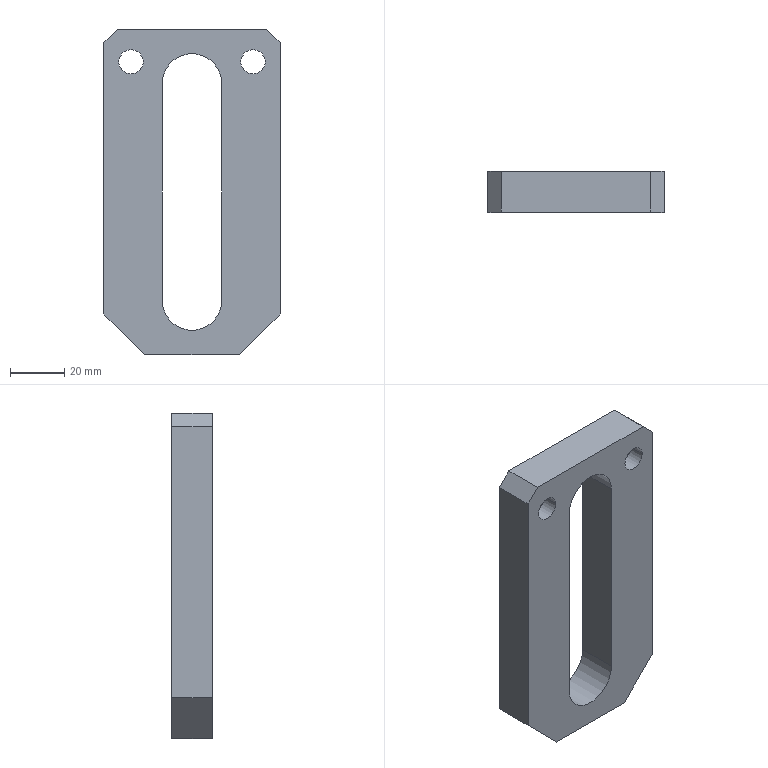Part | NX | features 001 2 | 1 solid | 24 faces | box 65 x 15 x 120 mm | volume 77204 mm3 | plane 14 | cylinder 10 | commonest cylinder face diameters 9 x4 15 x4 22 x2
STEP:
#1=CARTESIAN_POINT('',(114.773,73.,14.));
#2=VERTEX_POINT('',#1);
#3=CARTESIAN_POINT('',(114.773,58.,14.));
#4=VERTEX_POINT('',#3);
#5=CARTESIAN_POINT('',(114.773,73.,14.));
#6=DIRECTION('',(0.,-1.,0.));
#7=VECTOR('',#6,1000.);
#8=LINE('',#5,#7);
#9=EDGE_CURVE('',#2,#4,#8,.T.);
#10=ORIENTED_EDGE('',*,*,#9,.F.);
#11=CARTESIAN_POINT('',(114.773,73.,-66.));
#12=VERTEX_POINT('',#11);
#13=CARTESIAN_POINT('',(114.773,73.,-66.));
#14=DIRECTION('',(0.,0.,1.));
#15=VECTOR('',#14,1000.);
#16=LINE('',#13,#15);
#17=EDGE_CURVE('',#12,#2,#16,.T.);
#18=ORIENTED_EDGE('',*,*,#17,.F.);
#19=CARTESIAN_POINT('',(114.773,58.,-66.));
#20=VERTEX_POINT('',#19);
#21=CARTESIAN_POINT('',(114.773,58.,-66.));
#22=DIRECTION('',(0.,1.,0.));
#23=VECTOR('',#22,1000.);
#24=LINE('',#21,#23);
#25=EDGE_CURVE('',#20,#12,#24,.T.);
#26=ORIENTED_EDGE('',*,*,#25,.F.);
#27=CARTESIAN_POINT('',(114.773,58.,-66.));
#28=DIRECTION('',(0.,0.,1.));
#29=VECTOR('',#28,1000.);
#30=LINE('',#27,#29);
#31=EDGE_CURVE('',#20,#4,#30,.T.);
#32=ORIENTED_EDGE('',*,*,#31,.T.);
#33=EDGE_LOOP('',(#10,#18,#26,#32));
#34=FACE_BOUND('',#33,.T.);
#35=CARTESIAN_POINT('',(114.773,73.,-66.));
#36=DIRECTION('',(-1.,0.,0.));
#37=DIRECTION('',(0.,-1.,0.));
#38=AXIS2_PLACEMENT_3D('',#35,#36,#37);
#39=PLANE('',#38);
#40=ADVANCED_FACE('',(#34),#39,.T.);
#41=CARTESIAN_POINT('',(92.773,58.,14.));
#42=VERTEX_POINT('',#41);
#43=CARTESIAN_POINT('',(92.773,73.,14.));
#44=VERTEX_POINT('',#43);
#45=CARTESIAN_POINT('',(92.773,58.,14.));
#46=DIRECTION('',(0.,1.,0.));
#47=VECTOR('',#46,1000.);
#48=LINE('',#45,#47);
#49=EDGE_CURVE('',#42,#44,#48,.T.);
#50=ORIENTED_EDGE('',*,*,#49,.T.);
#51=CARTESIAN_POINT('',(103.773,73.,14.));
#52=DIRECTION('',(0.,-1.,0.));
#53=DIRECTION('',(1.,0.,0.));
#54=AXIS2_PLACEMENT_3D('',#51,#52,#53);
#55=CIRCLE('',#54,11.);
#56=EDGE_CURVE('',#2,#44,#55,.T.);
#57=ORIENTED_EDGE('',*,*,#56,.F.);
#58=ORIENTED_EDGE('',*,*,#9,.T.);
#59=CARTESIAN_POINT('',(103.773,58.,14.));
#60=DIRECTION('',(0.,1.,0.));
#61=DIRECTION('',(-1.,0.,0.));
#62=AXIS2_PLACEMENT_3D('',#59,#60,#61);
#63=CIRCLE('',#62,11.);
#64=EDGE_CURVE('',#42,#4,#63,.T.);
#65=ORIENTED_EDGE('',*,*,#64,.F.);
#66=EDGE_LOOP('',(#50,#57,#58,#65));
#67=FACE_BOUND('',#66,.T.);
#68=CARTESIAN_POINT('',(103.773,73.,14.));
#69=DIRECTION('',(0.,-1.,0.));
#70=DIRECTION('',(1.,0.,0.));
#71=AXIS2_PLACEMENT_3D('',#68,#69,#70);
#72=CYLINDRICAL_SURFACE('',#71,11.);
#73=ADVANCED_FACE('',(#67),#72,.F.);
#74=CARTESIAN_POINT('',(92.773,73.,-66.));
#75=VERTEX_POINT('',#74);
#76=CARTESIAN_POINT('',(92.773,58.,-66.));
#77=VERTEX_POINT('',#76);
#78=CARTESIAN_POINT('',(92.773,73.,-66.));
#79=DIRECTION('',(0.,-1.,0.));
#80=VECTOR('',#79,1000.);
#81=LINE('',#78,#80);
#82=EDGE_CURVE('',#75,#77,#81,.T.);
#83=ORIENTED_EDGE('',*,*,#82,.F.);
#84=CARTESIAN_POINT('',(92.773,73.,14.));
#85=DIRECTION('',(0.,0.,-1.));
#86=VECTOR('',#85,1000.);
#87=LINE('',#84,#86);
#88=EDGE_CURVE('',#44,#75,#87,.T.);
#89=ORIENTED_EDGE('',*,*,#88,.F.);
#90=ORIENTED_EDGE('',*,*,#49,.F.);
#91=CARTESIAN_POINT('',(92.773,58.,14.));
#92=DIRECTION('',(0.,0.,-1.));
#93=VECTOR('',#92,1000.);
#94=LINE('',#91,#93);
#95=EDGE_CURVE('',#42,#77,#94,.T.);
#96=ORIENTED_EDGE('',*,*,#95,.T.);
#97=EDGE_LOOP('',(#83,#89,#90,#96));
#98=FACE_BOUND('',#97,.T.);
#99=CARTESIAN_POINT('',(92.773,73.,-66.));
#100=DIRECTION('',(1.,0.,0.));
#101=DIRECTION('',(0.,1.,0.));
#102=AXIS2_PLACEMENT_3D('',#99,#100,#101);
#103=PLANE('',#102);
#104=ADVANCED_FACE('',(#98),#103,.T.);
#105=ORIENTED_EDGE('',*,*,#25,.T.);
#106=CARTESIAN_POINT('',(103.773,73.,-66.));
#107=DIRECTION('',(0.,-1.,0.));
#108=DIRECTION('',(-1.,0.,0.));
#109=AXIS2_PLACEMENT_3D('',#106,#107,#108);
#110=CIRCLE('',#109,11.);
#111=EDGE_CURVE('',#75,#12,#110,.T.);
#112=ORIENTED_EDGE('',*,*,#111,.F.);
#113=ORIENTED_EDGE('',*,*,#82,.T.);
#114=CARTESIAN_POINT('',(103.773,58.,-66.));
#115=DIRECTION('',(0.,1.,0.));
#116=DIRECTION('',(1.,0.,0.));
#117=AXIS2_PLACEMENT_3D('',#114,#115,#116);
#118=CIRCLE('',#117,11.);
#119=EDGE_CURVE('',#20,#77,#118,.T.);
#120=ORIENTED_EDGE('',*,*,#119,.F.);
#121=EDGE_LOOP('',(#105,#112,#113,#120));
#122=FACE_BOUND('',#121,.T.);
#123=CARTESIAN_POINT('',(103.773,73.,-66.));
#124=DIRECTION('',(0.,-1.,0.));
#125=DIRECTION('',(1.,0.,0.));
#126=AXIS2_PLACEMENT_3D('',#123,#124,#125);
#127=CYLINDRICAL_SURFACE('',#126,11.);
#128=ADVANCED_FACE('',(#122),#127,.F.);
#129=CARTESIAN_POINT('',(88.773,64.,22.));
#130=VERTEX_POINT('',#129);
#131=CARTESIAN_POINT('',(88.773,73.,22.));
#132=VERTEX_POINT('',#131);
#133=CARTESIAN_POINT('',(88.773,73.,22.));
#134=DIRECTION('',(0.,-1.,0.));
#135=VECTOR('',#134,1000.);
#136=LINE('',#133,#135);
#137=EDGE_CURVE('',#130,#132,#136,.F.);
#138=ORIENTED_EDGE('',*,*,#137,.T.);
#139=CARTESIAN_POINT('',(73.773,73.,22.));
#140=VERTEX_POINT('',#139);
#141=CARTESIAN_POINT('',(81.273,73.,22.));
#142=DIRECTION('',(0.,-1.,0.));
#143=DIRECTION('',(-1.,0.,0.));
#144=AXIS2_PLACEMENT_3D('',#141,#142,#143);
#145=CIRCLE('',#144,7.5);
#146=EDGE_CURVE('',#140,#132,#145,.T.);
#147=ORIENTED_EDGE('',*,*,#146,.F.);
#148=CARTESIAN_POINT('',(73.773,64.,22.));
#149=VERTEX_POINT('',#148);
#150=CARTESIAN_POINT('',(73.773,73.,22.));
#151=DIRECTION('',(0.,-1.,0.));
#152=VECTOR('',#151,1000.);
#153=LINE('',#150,#152);
#154=EDGE_CURVE('',#140,#149,#153,.T.);
#155=ORIENTED_EDGE('',*,*,#154,.T.);
#156=CARTESIAN_POINT('',(81.273,64.,22.));
#157=DIRECTION('',(0.,1.,0.));
#158=DIRECTION('',(1.,0.,0.));
#159=AXIS2_PLACEMENT_3D('',#156,#157,#158);
#160=CIRCLE('',#159,7.5);
#161=EDGE_CURVE('',#130,#149,#160,.T.);
#162=ORIENTED_EDGE('',*,*,#161,.F.);
#163=EDGE_LOOP('',(#138,#147,#155,#162));
#164=FACE_BOUND('',#163,.T.);
#165=CARTESIAN_POINT('',(81.273,73.,22.));
#166=DIRECTION('',(0.,1.,0.));
#167=DIRECTION('',(-1.,0.,0.));
#168=AXIS2_PLACEMENT_3D('',#165,#166,#167);
#169=CYLINDRICAL_SURFACE('',#168,7.5);
#170=ADVANCED_FACE('',(#164),#169,.F.);
#171=CARTESIAN_POINT('',(81.273,64.,22.));
#172=DIRECTION('',(0.,1.,0.));
#173=DIRECTION('',(-1.,0.,0.));
#174=AXIS2_PLACEMENT_3D('',#171,#172,#173);
#175=CIRCLE('',#174,7.5);
#176=EDGE_CURVE('',#149,#130,#175,.T.);
#177=ORIENTED_EDGE('',*,*,#176,.F.);
#178=ORIENTED_EDGE('',*,*,#154,.F.);
#179=CARTESIAN_POINT('',(81.273,73.,22.));
#180=DIRECTION('',(0.,-1.,0.));
#181=DIRECTION('',(1.,0.,0.));
#182=AXIS2_PLACEMENT_3D('',#179,#180,#181);
#183=CIRCLE('',#182,7.5);
#184=EDGE_CURVE('',#132,#140,#183,.T.);
#185=ORIENTED_EDGE('',*,*,#184,.F.);
#186=ORIENTED_EDGE('',*,*,#137,.F.);
#187=EDGE_LOOP('',(#177,#178,#185,#186));
#188=FACE_BOUND('',#187,.T.);
#189=CARTESIAN_POINT('',(81.273,73.,22.));
#190=DIRECTION('',(0.,1.,0.));
#191=DIRECTION('',(-1.,0.,0.));
#192=AXIS2_PLACEMENT_3D('',#189,#190,#191);
#193=CYLINDRICAL_SURFACE('',#192,7.5);
#194=ADVANCED_FACE('',(#188),#193,.F.);
#195=CARTESIAN_POINT('',(76.773,64.,22.));
#196=VERTEX_POINT('',#195);
#197=CARTESIAN_POINT('',(85.773,64.,22.));
#198=VERTEX_POINT('',#197);
#199=CARTESIAN_POINT('',(81.273,64.,22.));
#200=DIRECTION('',(0.,-1.,0.));
#201=DIRECTION('',(-1.,0.,0.));
#202=AXIS2_PLACEMENT_3D('',#199,#200,#201);
#203=CIRCLE('',#202,4.5);
#204=EDGE_CURVE('',#196,#198,#203,.T.);
#205=ORIENTED_EDGE('',*,*,#204,.T.);
#206=CARTESIAN_POINT('',(81.273,64.,22.));
#207=DIRECTION('',(0.,-1.,0.));
#208=DIRECTION('',(1.,0.,0.));
#209=AXIS2_PLACEMENT_3D('',#206,#207,#208);
#210=CIRCLE('',#209,4.5);
#211=EDGE_CURVE('',#198,#196,#210,.T.);
#212=ORIENTED_EDGE('',*,*,#211,.T.);
#213=EDGE_LOOP('',(#205,#212));
#214=FACE_BOUND('',#213,.T.);
#215=ORIENTED_EDGE('',*,*,#161,.T.);
#216=ORIENTED_EDGE('',*,*,#176,.T.);
#217=EDGE_LOOP('',(#215,#216));
#218=FACE_BOUND('',#217,.T.);
#219=CARTESIAN_POINT('',(76.773,64.,22.));
#220=DIRECTION('',(0.,-1.,0.));
#221=DIRECTION('',(1.,0.,0.));
#222=AXIS2_PLACEMENT_3D('',#219,#220,#221);
#223=PLANE('',#222);
#224=ADVANCED_FACE('',(#214,#218),#223,.F.);
#225=CARTESIAN_POINT('',(85.773,58.,22.));
#226=VERTEX_POINT('',#225);
#227=CARTESIAN_POINT('',(85.773,64.,22.));
#228=DIRECTION('',(0.,-1.,0.));
#229=VECTOR('',#228,1000.);
#230=LINE('',#227,#229);
#231=EDGE_CURVE('',#226,#198,#230,.F.);
#232=ORIENTED_EDGE('',*,*,#231,.T.);
#233=ORIENTED_EDGE('',*,*,#204,.F.);
#234=CARTESIAN_POINT('',(76.773,58.,22.));
#235=VERTEX_POINT('',#234);
#236=CARTESIAN_POINT('',(76.773,64.,22.));
#237=DIRECTION('',(0.,-1.,0.));
#238=VECTOR('',#237,1000.);
#239=LINE('',#236,#238);
#240=EDGE_CURVE('',#196,#235,#239,.T.);
#241=ORIENTED_EDGE('',*,*,#240,.T.);
#242=CARTESIAN_POINT('',(81.273,58.,22.));
#243=DIRECTION('',(0.,1.,0.));
#244=DIRECTION('',(1.,0.,0.));
#245=AXIS2_PLACEMENT_3D('',#242,#243,#244);
#246=CIRCLE('',#245,4.5);
#247=EDGE_CURVE('',#226,#235,#246,.T.);
#248=ORIENTED_EDGE('',*,*,#247,.F.);
#249=EDGE_LOOP('',(#232,#233,#241,#248));
#250=FACE_BOUND('',#249,.T.);
#251=CARTESIAN_POINT('',(81.273,73.,22.));
#252=DIRECTION('',(0.,1.,0.));
#253=DIRECTION('',(-1.,0.,0.));
#254=AXIS2_PLACEMENT_3D('',#251,#252,#253);
#255=CYLINDRICAL_SURFACE('',#254,4.5);
#256=ADVANCED_FACE('',(#250),#255,.F.);
#257=CARTESIAN_POINT('',(81.273,58.,22.));
#258=DIRECTION('',(0.,1.,0.));
#259=DIRECTION('',(-1.,0.,0.));
#260=AXIS2_PLACEMENT_3D('',#257,#258,#259);
#261=CIRCLE('',#260,4.5);
#262=EDGE_CURVE('',#235,#226,#261,.T.);
#263=ORIENTED_EDGE('',*,*,#262,.F.);
#264=ORIENTED_EDGE('',*,*,#240,.F.);
#265=ORIENTED_EDGE('',*,*,#211,.F.);
#266=ORIENTED_EDGE('',*,*,#231,.F.);
#267=EDGE_LOOP('',(#263,#264,#265,#266));
#268=FACE_BOUND('',#267,.T.);
#269=CARTESIAN_POINT('',(81.273,73.,22.));
#270=DIRECTION('',(0.,1.,0.));
#271=DIRECTION('',(-1.,0.,0.));
#272=AXIS2_PLACEMENT_3D('',#269,#270,#271);
#273=CYLINDRICAL_SURFACE('',#272,4.5);
#274=ADVANCED_FACE('',(#268),#273,.F.);
#275=CARTESIAN_POINT('',(130.773,58.,22.));
#276=VERTEX_POINT('',#275);
#277=CARTESIAN_POINT('',(130.773,64.,22.));
#278=VERTEX_POINT('',#277);
#279=CARTESIAN_POINT('',(130.773,64.,22.));
#280=DIRECTION('',(0.,-1.,0.));
#281=VECTOR('',#280,1000.);
#282=LINE('',#279,#281);
#283=EDGE_CURVE('',#276,#278,#282,.F.);
#284=ORIENTED_EDGE('',*,*,#283,.T.);
#285=CARTESIAN_POINT('',(121.773,64.,22.));
#286=VERTEX_POINT('',#285);
#287=CARTESIAN_POINT('',(126.273,64.,22.));
#288=DIRECTION('',(0.,-1.,0.));
#289=DIRECTION('',(-1.,0.,0.));
#290=AXIS2_PLACEMENT_3D('',#287,#288,#289);
#291=CIRCLE('',#290,4.5);
#292=EDGE_CURVE('',#286,#278,#291,.T.);
#293=ORIENTED_EDGE('',*,*,#292,.F.);
#294=CARTESIAN_POINT('',(121.773,58.,22.));
#295=VERTEX_POINT('',#294);
#296=CARTESIAN_POINT('',(121.773,64.,22.));
#297=DIRECTION('',(0.,-1.,0.));
#298=VECTOR('',#297,1000.);
#299=LINE('',#296,#298);
#300=EDGE_CURVE('',#286,#295,#299,.T.);
#301=ORIENTED_EDGE('',*,*,#300,.T.);
#302=CARTESIAN_POINT('',(126.273,58.,22.));
#303=DIRECTION('',(0.,1.,0.));
#304=DIRECTION('',(1.,0.,0.));
#305=AXIS2_PLACEMENT_3D('',#302,#303,#304);
#306=CIRCLE('',#305,4.5);
#307=EDGE_CURVE('',#276,#295,#306,.T.);
#308=ORIENTED_EDGE('',*,*,#307,.F.);
#309=EDGE_LOOP('',(#284,#293,#301,#308));
#310=FACE_BOUND('',#309,.T.);
#311=CARTESIAN_POINT('',(126.273,73.,22.));
#312=DIRECTION('',(0.,1.,0.));
#313=DIRECTION('',(-1.,0.,0.));
#314=AXIS2_PLACEMENT_3D('',#311,#312,#313);
#315=CYLINDRICAL_SURFACE('',#314,4.5);
#316=ADVANCED_FACE('',(#310),#315,.F.);
#317=CARTESIAN_POINT('',(126.273,58.,22.));
#318=DIRECTION('',(0.,1.,0.));
#319=DIRECTION('',(-1.,0.,0.));
#320=AXIS2_PLACEMENT_3D('',#317,#318,#319);
#321=CIRCLE('',#320,4.5);
#322=EDGE_CURVE('',#295,#276,#321,.T.);
#323=ORIENTED_EDGE('',*,*,#322,.F.);
#324=ORIENTED_EDGE('',*,*,#300,.F.);
#325=CARTESIAN_POINT('',(126.273,64.,22.));
#326=DIRECTION('',(0.,-1.,0.));
#327=DIRECTION('',(1.,0.,0.));
#328=AXIS2_PLACEMENT_3D('',#325,#326,#327);
#329=CIRCLE('',#328,4.5);
#330=EDGE_CURVE('',#278,#286,#329,.T.);
#331=ORIENTED_EDGE('',*,*,#330,.F.);
#332=ORIENTED_EDGE('',*,*,#283,.F.);
#333=EDGE_LOOP('',(#323,#324,#331,#332));
#334=FACE_BOUND('',#333,.T.);
#335=CARTESIAN_POINT('',(126.273,73.,22.));
#336=DIRECTION('',(0.,1.,0.));
#337=DIRECTION('',(-1.,0.,0.));
#338=AXIS2_PLACEMENT_3D('',#335,#336,#337);
#339=CYLINDRICAL_SURFACE('',#338,4.5);
#340=ADVANCED_FACE('',(#334),#339,.F.);
#341=CARTESIAN_POINT('',(131.273,73.,34.));
#342=VERTEX_POINT('',#341);
#343=CARTESIAN_POINT('',(131.273,58.,34.));
#344=VERTEX_POINT('',#343);
#345=CARTESIAN_POINT('',(131.273,73.,34.));
#346=DIRECTION('',(0.,-1.,0.));
#347=VECTOR('',#346,1000.);
#348=LINE('',#345,#347);
#349=EDGE_CURVE('',#342,#344,#348,.T.);
#350=ORIENTED_EDGE('',*,*,#349,.T.);
#351=CARTESIAN_POINT('',(136.273,58.,29.));
#352=VERTEX_POINT('',#351);
#353=CARTESIAN_POINT('',(136.273,58.,29.));
#354=DIRECTION('',(-0.7071,0.,0.7071));
#355=VECTOR('',#354,1000.);
#356=LINE('',#353,#355);
#357=EDGE_CURVE('',#352,#344,#356,.T.);
#358=ORIENTED_EDGE('',*,*,#357,.F.);
#359=CARTESIAN_POINT('',(136.273,73.,29.));
#360=VERTEX_POINT('',#359);
#361=CARTESIAN_POINT('',(136.273,58.,29.));
#362=DIRECTION('',(0.,1.,0.));
#363=VECTOR('',#362,1000.);
#364=LINE('',#361,#363);
#365=EDGE_CURVE('',#352,#360,#364,.T.);
#366=ORIENTED_EDGE('',*,*,#365,.T.);
#367=CARTESIAN_POINT('',(131.273,73.,34.));
#368=DIRECTION('',(0.7071,0.,-0.7071));
#369=VECTOR('',#368,1000.);
#370=LINE('',#367,#369);
#371=EDGE_CURVE('',#342,#360,#370,.T.);
#372=ORIENTED_EDGE('',*,*,#371,.F.);
#373=EDGE_LOOP('',(#350,#358,#366,#372));
#374=FACE_BOUND('',#373,.T.);
#375=CARTESIAN_POINT('',(136.273,73.,29.));
#376=DIRECTION('',(-0.7071,0.,-0.7071));
#377=DIRECTION('',(0.,-1.,0.));
#378=AXIS2_PLACEMENT_3D('',#375,#376,#377);
#379=PLANE('',#378);
#380=ADVANCED_FACE('',(#374),#379,.F.);
#381=CARTESIAN_POINT('',(71.273,73.,29.));
#382=VERTEX_POINT('',#381);
#383=CARTESIAN_POINT('',(71.273,58.,29.));
#384=VERTEX_POINT('',#383);
#385=CARTESIAN_POINT('',(71.273,73.,29.));
#386=DIRECTION('',(0.,-1.,0.));
#387=VECTOR('',#386,1000.);
#388=LINE('',#385,#387);
#389=EDGE_CURVE('',#382,#384,#388,.T.);
#390=ORIENTED_EDGE('',*,*,#389,.T.);
#391=CARTESIAN_POINT('',(76.273,58.,34.));
#392=VERTEX_POINT('',#391);
#393=CARTESIAN_POINT('',(76.273,58.,34.));
#394=DIRECTION('',(-0.7071,0.,-0.7071));
#395=VECTOR('',#394,1000.);
#396=LINE('',#393,#395);
#397=EDGE_CURVE('',#392,#384,#396,.T.);
#398=ORIENTED_EDGE('',*,*,#397,.F.);
#399=CARTESIAN_POINT('',(76.273,73.,34.));
#400=VERTEX_POINT('',#399);
#401=CARTESIAN_POINT('',(76.273,58.,34.));
#402=DIRECTION('',(0.,1.,0.));
#403=VECTOR('',#402,1000.);
#404=LINE('',#401,#403);
#405=EDGE_CURVE('',#392,#400,#404,.T.);
#406=ORIENTED_EDGE('',*,*,#405,.T.);
#407=CARTESIAN_POINT('',(71.273,73.,29.));
#408=DIRECTION('',(0.7071,0.,0.7071));
#409=VECTOR('',#408,1000.);
#410=LINE('',#407,#409);
#411=EDGE_CURVE('',#382,#400,#410,.T.);
#412=ORIENTED_EDGE('',*,*,#411,.F.);
#413=EDGE_LOOP('',(#390,#398,#406,#412));
#414=FACE_BOUND('',#413,.T.);
#415=CARTESIAN_POINT('',(76.273,73.,34.));
#416=DIRECTION('',(0.7071,0.,-0.7071));
#417=DIRECTION('',(0.,-1.,0.));
#418=AXIS2_PLACEMENT_3D('',#415,#416,#417);
#419=PLANE('',#418);
#420=ADVANCED_FACE('',(#414),#419,.F.);
#421=ORIENTED_EDGE('',*,*,#389,.F.);
#422=CARTESIAN_POINT('',(71.273,73.,-71.));
#423=VERTEX_POINT('',#422);
#424=CARTESIAN_POINT('',(71.273,73.,29.));
#425=DIRECTION('',(0.,0.,-1.));
#426=VECTOR('',#425,1000.);
#427=LINE('',#424,#426);
#428=EDGE_CURVE('',#382,#423,#427,.T.);
#429=ORIENTED_EDGE('',*,*,#428,.T.);
#430=CARTESIAN_POINT('',(71.273,58.,-71.));
#431=VERTEX_POINT('',#430);
#432=CARTESIAN_POINT('',(71.273,58.,-71.));
#433=DIRECTION('',(0.,1.,0.));
#434=VECTOR('',#433,1000.);
#435=LINE('',#432,#434);
#436=EDGE_CURVE('',#431,#423,#435,.T.);
#437=ORIENTED_EDGE('',*,*,#436,.F.);
#438=CARTESIAN_POINT('',(71.273,58.,29.));
#439=DIRECTION('',(0.,0.,-1.));
#440=VECTOR('',#439,1000.);
#441=LINE('',#438,#440);
#442=EDGE_CURVE('',#384,#431,#441,.T.);
#443=ORIENTED_EDGE('',*,*,#442,.F.);
#444=EDGE_LOOP('',(#421,#429,#437,#443));
#445=FACE_BOUND('',#444,.T.);
#446=CARTESIAN_POINT('',(71.273,73.,-86.));
#447=DIRECTION('',(1.,0.,0.));
#448=DIRECTION('',(0.,1.,0.));
#449=AXIS2_PLACEMENT_3D('',#446,#447,#448);
#450=PLANE('',#449);
#451=ADVANCED_FACE('',(#445),#450,.F.);
#452=CARTESIAN_POINT('',(86.273,73.,-86.));
#453=VERTEX_POINT('',#452);
#454=CARTESIAN_POINT('',(86.273,58.,-86.));
#455=VERTEX_POINT('',#454);
#456=CARTESIAN_POINT('',(86.273,73.,-86.));
#457=DIRECTION('',(0.,-1.,0.));
#458=VECTOR('',#457,1000.);
#459=LINE('',#456,#458);
#460=EDGE_CURVE('',#453,#455,#459,.T.);
#461=ORIENTED_EDGE('',*,*,#460,.T.);
#462=CARTESIAN_POINT('',(71.273,58.,-71.));
#463=DIRECTION('',(0.7071,0.,-0.7071));
#464=VECTOR('',#463,1000.);
#465=LINE('',#462,#464);
#466=EDGE_CURVE('',#431,#455,#465,.T.);
#467=ORIENTED_EDGE('',*,*,#466,.F.);
#468=ORIENTED_EDGE('',*,*,#436,.T.);
#469=CARTESIAN_POINT('',(86.273,73.,-86.));
#470=DIRECTION('',(-0.7071,0.,0.7071));
#471=VECTOR('',#470,1000.);
#472=LINE('',#469,#471);
#473=EDGE_CURVE('',#453,#423,#472,.T.);
#474=ORIENTED_EDGE('',*,*,#473,.F.);
#475=EDGE_LOOP('',(#461,#467,#468,#474));
#476=FACE_BOUND('',#475,.T.);
#477=CARTESIAN_POINT('',(71.273,73.,-71.));
#478=DIRECTION('',(0.7071,0.,0.7071));
#479=DIRECTION('',(0.,-1.,0.));
#480=AXIS2_PLACEMENT_3D('',#477,#478,#479);
#481=PLANE('',#480);
#482=ADVANCED_FACE('',(#476),#481,.F.);
#483=ORIENTED_EDGE('',*,*,#460,.F.);
#484=CARTESIAN_POINT('',(121.273,73.,-86.));
#485=VERTEX_POINT('',#484);
#486=CARTESIAN_POINT('',(86.273,73.,-86.));
#487=DIRECTION('',(1.,0.,0.));
#488=VECTOR('',#487,1000.);
#489=LINE('',#486,#488);
#490=EDGE_CURVE('',#453,#485,#489,.T.);
#491=ORIENTED_EDGE('',*,*,#490,.T.);
#492=CARTESIAN_POINT('',(121.273,58.,-86.));
#493=VERTEX_POINT('',#492);
#494=CARTESIAN_POINT('',(121.273,58.,-86.));
#495=DIRECTION('',(0.,1.,0.));
#496=VECTOR('',#495,1000.);
#497=LINE('',#494,#496);
#498=EDGE_CURVE('',#493,#485,#497,.T.);
#499=ORIENTED_EDGE('',*,*,#498,.F.);
#500=CARTESIAN_POINT('',(86.273,58.,-86.));
#501=DIRECTION('',(1.,0.,0.));
#502=VECTOR('',#501,1000.);
#503=LINE('',#500,#502);
#504=EDGE_CURVE('',#455,#493,#503,.T.);
#505=ORIENTED_EDGE('',*,*,#504,.F.);
#506=EDGE_LOOP('',(#483,#491,#499,#505));
#507=FACE_BOUND('',#506,.T.);
#508=CARTESIAN_POINT('',(71.273,73.,-86.));
#509=DIRECTION('',(0.,0.,1.));
#510=DIRECTION('',(1.,0.,0.));
#511=AXIS2_PLACEMENT_3D('',#508,#509,#510);
#512=PLANE('',#511);
#513=ADVANCED_FACE('',(#507),#512,.F.);
#514=CARTESIAN_POINT('',(136.273,73.,-71.));
#515=VERTEX_POINT('',#514);
#516=CARTESIAN_POINT('',(136.273,58.,-71.));
#517=VERTEX_POINT('',#516);
#518=CARTESIAN_POINT('',(136.273,73.,-71.));
#519=DIRECTION('',(0.,-1.,0.));
#520=VECTOR('',#519,1000.);
#521=LINE('',#518,#520);
#522=EDGE_CURVE('',#515,#517,#521,.T.);
#523=ORIENTED_EDGE('',*,*,#522,.T.);
#524=CARTESIAN_POINT('',(121.273,58.,-86.));
#525=DIRECTION('',(0.7071,0.,0.7071));
#526=VECTOR('',#525,1000.);
#527=LINE('',#524,#526);
#528=EDGE_CURVE('',#493,#517,#527,.T.);
#529=ORIENTED_EDGE('',*,*,#528,.F.);
#530=ORIENTED_EDGE('',*,*,#498,.T.);
#531=CARTESIAN_POINT('',(136.273,73.,-71.));
#532=DIRECTION('',(-0.7071,0.,-0.7071));
#533=VECTOR('',#532,1000.);
#534=LINE('',#531,#533);
#535=EDGE_CURVE('',#515,#485,#534,.T.);
#536=ORIENTED_EDGE('',*,*,#535,.F.);
#537=EDGE_LOOP('',(#523,#529,#530,#536));
#538=FACE_BOUND('',#537,.T.);
#539=CARTESIAN_POINT('',(121.273,73.,-86.));
#540=DIRECTION('',(-0.7071,0.,0.7071));
#541=DIRECTION('',(0.,-1.,0.));
#542=AXIS2_PLACEMENT_3D('',#539,#540,#541);
#543=PLANE('',#542);
#544=ADVANCED_FACE('',(#538),#543,.F.);
#545=ORIENTED_EDGE('',*,*,#365,.F.);
#546=CARTESIAN_POINT('',(136.273,58.,-71.));
#547=DIRECTION('',(0.,0.,1.));
#548=VECTOR('',#547,1000.);
#549=LINE('',#546,#548);
#550=EDGE_CURVE('',#517,#352,#549,.T.);
#551=ORIENTED_EDGE('',*,*,#550,.F.);
#552=ORIENTED_EDGE('',*,*,#522,.F.);
#553=CARTESIAN_POINT('',(136.273,73.,-71.));
#554=DIRECTION('',(0.,0.,1.));
#555=VECTOR('',#554,1000.);
#556=LINE('',#553,#555);
#557=EDGE_CURVE('',#515,#360,#556,.T.);
#558=ORIENTED_EDGE('',*,*,#557,.T.);
#559=EDGE_LOOP('',(#545,#551,#552,#558));
#560=FACE_BOUND('',#559,.T.);
#561=CARTESIAN_POINT('',(136.273,73.,-86.));
#562=DIRECTION('',(-1.,0.,0.));
#563=DIRECTION('',(0.,-1.,0.));
#564=AXIS2_PLACEMENT_3D('',#561,#562,#563);
#565=PLANE('',#564);
#566=ADVANCED_FACE('',(#560),#565,.F.);
#567=ORIENTED_EDGE('',*,*,#95,.F.);
#568=ORIENTED_EDGE('',*,*,#64,.T.);
#569=ORIENTED_EDGE('',*,*,#31,.F.);
#570=ORIENTED_EDGE('',*,*,#119,.T.);
#571=EDGE_LOOP('',(#567,#568,#569,#570));
#572=FACE_BOUND('',#571,.T.);
#573=ORIENTED_EDGE('',*,*,#247,.T.);
#574=ORIENTED_EDGE('',*,*,#262,.T.);
#575=EDGE_LOOP('',(#573,#574));
#576=FACE_BOUND('',#575,.T.);
#577=ORIENTED_EDGE('',*,*,#307,.T.);
#578=ORIENTED_EDGE('',*,*,#322,.T.);
#579=EDGE_LOOP('',(#577,#578));
#580=FACE_BOUND('',#579,.T.);
#581=ORIENTED_EDGE('',*,*,#357,.T.);
#582=CARTESIAN_POINT('',(131.273,58.,34.));
#583=DIRECTION('',(-1.,0.,0.));
#584=VECTOR('',#583,1000.);
#585=LINE('',#582,#584);
#586=EDGE_CURVE('',#344,#392,#585,.T.);
#587=ORIENTED_EDGE('',*,*,#586,.T.);
#588=ORIENTED_EDGE('',*,*,#397,.T.);
#589=ORIENTED_EDGE('',*,*,#442,.T.);
#590=ORIENTED_EDGE('',*,*,#466,.T.);
#591=ORIENTED_EDGE('',*,*,#504,.T.);
#592=ORIENTED_EDGE('',*,*,#528,.T.);
#593=ORIENTED_EDGE('',*,*,#550,.T.);
#594=EDGE_LOOP('',(#581,#587,#588,#589,#590,#591,#592,#593));
#595=FACE_BOUND('',#594,.T.);
#596=CARTESIAN_POINT('',(103.773,58.,-26.));
#597=DIRECTION('',(0.,1.,0.));
#598=DIRECTION('',(-1.,0.,0.));
#599=AXIS2_PLACEMENT_3D('',#596,#597,#598);
#600=PLANE('',#599);
#601=ADVANCED_FACE('',(#572,#576,#580,#595),#600,.F.);
#602=ORIENTED_EDGE('',*,*,#349,.F.);
#603=CARTESIAN_POINT('',(131.273,73.,34.));
#604=DIRECTION('',(-1.,0.,0.));
#605=VECTOR('',#604,1000.);
#606=LINE('',#603,#605);
#607=EDGE_CURVE('',#342,#400,#606,.T.);
#608=ORIENTED_EDGE('',*,*,#607,.T.);
#609=ORIENTED_EDGE('',*,*,#405,.F.);
#610=ORIENTED_EDGE('',*,*,#586,.F.);
#611=EDGE_LOOP('',(#602,#608,#609,#610));
#612=FACE_BOUND('',#611,.T.);
#613=CARTESIAN_POINT('',(71.273,73.,34.));
#614=DIRECTION('',(0.,0.,-1.));
#615=DIRECTION('',(-1.,0.,0.));
#616=AXIS2_PLACEMENT_3D('',#613,#614,#615);
#617=PLANE('',#616);
#618=ADVANCED_FACE('',(#612),#617,.F.);
#619=ORIENTED_EDGE('',*,*,#111,.T.);
#620=ORIENTED_EDGE('',*,*,#17,.T.);
#621=ORIENTED_EDGE('',*,*,#56,.T.);
#622=ORIENTED_EDGE('',*,*,#88,.T.);
#623=EDGE_LOOP('',(#619,#620,#621,#622));
#624=FACE_BOUND('',#623,.T.);
#625=ORIENTED_EDGE('',*,*,#146,.T.);
#626=ORIENTED_EDGE('',*,*,#184,.T.);
#627=EDGE_LOOP('',(#625,#626));
#628=FACE_BOUND('',#627,.T.);
#629=CARTESIAN_POINT('',(118.773,73.,22.));
#630=VERTEX_POINT('',#629);
#631=CARTESIAN_POINT('',(133.773,73.,22.));
#632=VERTEX_POINT('',#631);
#633=CARTESIAN_POINT('',(126.273,73.,22.));
#634=DIRECTION('',(0.,-1.,0.));
#635=DIRECTION('',(-1.,0.,0.));
#636=AXIS2_PLACEMENT_3D('',#633,#634,#635);
#637=CIRCLE('',#636,7.5);
#638=EDGE_CURVE('',#630,#632,#637,.T.);
#639=ORIENTED_EDGE('',*,*,#638,.T.);
#640=CARTESIAN_POINT('',(126.273,73.,22.));
#641=DIRECTION('',(0.,-1.,0.));
#642=DIRECTION('',(1.,0.,0.));
#643=AXIS2_PLACEMENT_3D('',#640,#641,#642);
#644=CIRCLE('',#643,7.5);
#645=EDGE_CURVE('',#632,#630,#644,.T.);
#646=ORIENTED_EDGE('',*,*,#645,.T.);
#647=EDGE_LOOP('',(#639,#646));
#648=FACE_BOUND('',#647,.T.);
#649=ORIENTED_EDGE('',*,*,#371,.T.);
#650=ORIENTED_EDGE('',*,*,#557,.F.);
#651=ORIENTED_EDGE('',*,*,#535,.T.);
#652=ORIENTED_EDGE('',*,*,#490,.F.);
#653=ORIENTED_EDGE('',*,*,#473,.T.);
#654=ORIENTED_EDGE('',*,*,#428,.F.);
#655=ORIENTED_EDGE('',*,*,#411,.T.);
#656=ORIENTED_EDGE('',*,*,#607,.F.);
#657=EDGE_LOOP('',(#649,#650,#651,#652,#653,#654,#655,#656));
#658=FACE_BOUND('',#657,.T.);
#659=CARTESIAN_POINT('',(103.773,73.,-26.));
#660=DIRECTION('',(0.,1.,0.));
#661=DIRECTION('',(-1.,0.,0.));
#662=AXIS2_PLACEMENT_3D('',#659,#660,#661);
#663=PLANE('',#662);
#664=ADVANCED_FACE('',(#624,#628,#648,#658),#663,.T.);
#665=CARTESIAN_POINT('',(118.773,64.,22.));
#666=VERTEX_POINT('',#665);
#667=CARTESIAN_POINT('',(133.773,64.,22.));
#668=VERTEX_POINT('',#667);
#669=CARTESIAN_POINT('',(126.273,64.,22.));
#670=DIRECTION('',(0.,1.,0.));
#671=DIRECTION('',(-1.,0.,0.));
#672=AXIS2_PLACEMENT_3D('',#669,#670,#671);
#673=CIRCLE('',#672,7.5);
#674=EDGE_CURVE('',#666,#668,#673,.T.);
#675=ORIENTED_EDGE('',*,*,#674,.F.);
#676=CARTESIAN_POINT('',(118.773,73.,22.));
#677=DIRECTION('',(0.,-1.,0.));
#678=VECTOR('',#677,1000.);
#679=LINE('',#676,#678);
#680=EDGE_CURVE('',#630,#666,#679,.T.);
#681=ORIENTED_EDGE('',*,*,#680,.F.);
#682=ORIENTED_EDGE('',*,*,#645,.F.);
#683=CARTESIAN_POINT('',(133.773,73.,22.));
#684=DIRECTION('',(0.,-1.,0.));
#685=VECTOR('',#684,1000.);
#686=LINE('',#683,#685);
#687=EDGE_CURVE('',#668,#632,#686,.F.);
#688=ORIENTED_EDGE('',*,*,#687,.F.);
#689=EDGE_LOOP('',(#675,#681,#682,#688));
#690=FACE_BOUND('',#689,.T.);
#691=CARTESIAN_POINT('',(126.273,73.,22.));
#692=DIRECTION('',(0.,1.,0.));
#693=DIRECTION('',(-1.,0.,0.));
#694=AXIS2_PLACEMENT_3D('',#691,#692,#693);
#695=CYLINDRICAL_SURFACE('',#694,7.5);
#696=ADVANCED_FACE('',(#690),#695,.F.);
#697=ORIENTED_EDGE('',*,*,#292,.T.);
#698=ORIENTED_EDGE('',*,*,#330,.T.);
#699=EDGE_LOOP('',(#697,#698));
#700=FACE_BOUND('',#699,.T.);
#701=CARTESIAN_POINT('',(126.273,64.,22.));
#702=DIRECTION('',(0.,1.,0.));
#703=DIRECTION('',(1.,0.,0.));
#704=AXIS2_PLACEMENT_3D('',#701,#702,#703);
#705=CIRCLE('',#704,7.5);
#706=EDGE_CURVE('',#668,#666,#705,.T.);
#707=ORIENTED_EDGE('',*,*,#706,.T.);
#708=ORIENTED_EDGE('',*,*,#674,.T.);
#709=EDGE_LOOP('',(#707,#708));
#710=FACE_BOUND('',#709,.T.);
#711=CARTESIAN_POINT('',(121.773,64.,22.));
#712=DIRECTION('',(0.,-1.,0.));
#713=DIRECTION('',(1.,0.,0.));
#714=AXIS2_PLACEMENT_3D('',#711,#712,#713);
#715=PLANE('',#714);
#716=ADVANCED_FACE('',(#700,#710),#715,.F.);
#717=ORIENTED_EDGE('',*,*,#687,.T.);
#718=ORIENTED_EDGE('',*,*,#638,.F.);
#719=ORIENTED_EDGE('',*,*,#680,.T.);
#720=ORIENTED_EDGE('',*,*,#706,.F.);
#721=EDGE_LOOP('',(#717,#718,#719,#720));
#722=FACE_BOUND('',#721,.T.);
#723=CARTESIAN_POINT('',(126.273,73.,22.));
#724=DIRECTION('',(0.,1.,0.));
#725=DIRECTION('',(-1.,0.,0.));
#726=AXIS2_PLACEMENT_3D('',#723,#724,#725);
#727=CYLINDRICAL_SURFACE('',#726,7.5);
#728=ADVANCED_FACE('',(#722),#727,.F.);
#729=CLOSED_SHELL('',(#40,#73,#104,#128,#170,#194,#224,#256,#274,#316,#340,#380,#420,#451,#482,#513,#544,#566,#601,#618,#664,#696,#716,#728));
#730=MANIFOLD_SOLID_BREP('',#729);
#731=(LENGTH_UNIT()NAMED_UNIT(*)SI_UNIT(.MILLI.,.METRE.));
#732=UNCERTAINTY_MEASURE_WITH_UNIT(LENGTH_MEASURE(0.00001),#731,'','');
#733=(NAMED_UNIT(*)PLANE_ANGLE_UNIT()SI_UNIT($,.RADIAN.));
#734=(NAMED_UNIT(*)SI_UNIT($,.STERADIAN.)SOLID_ANGLE_UNIT());
#735=(GEOMETRIC_REPRESENTATION_CONTEXT(3)GLOBAL_UNCERTAINTY_ASSIGNED_CONTEXT((#732))GLOBAL_UNIT_ASSIGNED_CONTEXT((#731,#733,#734))REPRESENTATION_CONTEXT('',''));
#736=ADVANCED_BREP_SHAPE_REPRESENTATION('',(#730),#735);